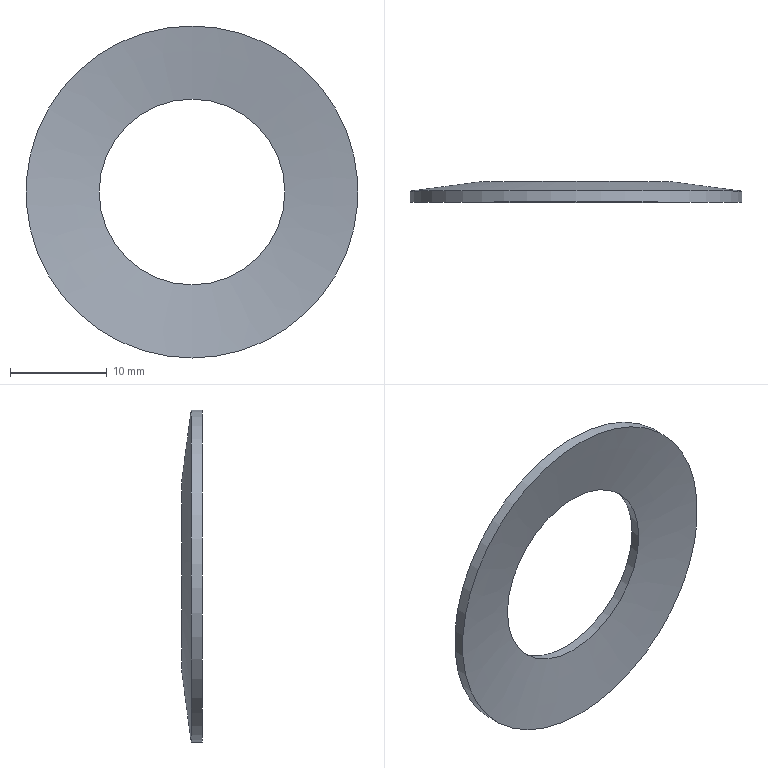Part | NX | features belleville 1.35in 2 | 1 solid | 4 faces | box 34.29 x 2.131 x 34.29 mm | volume 726.461 mm3 | cone 3 | cylinder 1 | commonest cylinder face diameters 34.29 x1
STEP:
#1=CARTESIAN_POINT('',(0.,0.2317,-17.145));
#2=VERTEX_POINT('',#1);
#3=CARTESIAN_POINT('',(0.,0.2317,0.));
#4=DIRECTION('',(0.,-1.,0.));
#5=DIRECTION('',(0.,0.,-1.));
#6=AXIS2_PLACEMENT_3D('',#3,#4,#5);
#7=CIRCLE('',#6,17.145);
#8=EDGE_CURVE('',#2,#2,#7,.F.);
#9=ORIENTED_EDGE('',*,*,#8,.F.);
#10=EDGE_LOOP('',(#9));
#11=FACE_BOUND('',#10,.T.);
#12=CARTESIAN_POINT('',(0.,1.229,-9.588));
#13=VERTEX_POINT('',#12);
#14=CARTESIAN_POINT('',(0.,1.229,0.));
#15=DIRECTION('',(0.,-1.,0.));
#16=DIRECTION('',(0.,0.,-1.));
#17=AXIS2_PLACEMENT_3D('',#14,#15,#16);
#18=CIRCLE('',#17,9.588);
#19=EDGE_CURVE('',#13,#13,#18,.T.);
#20=ORIENTED_EDGE('',*,*,#19,.F.);
#21=EDGE_LOOP('',(#20));
#22=FACE_BOUND('',#21,.T.);
#23=CARTESIAN_POINT('',(0.,1.229,0.));
#24=DIRECTION('',(0.,-1.,0.));
#25=DIRECTION('',(0.,0.,-1.));
#26=AXIS2_PLACEMENT_3D('',#23,#24,#25);
#27=CONICAL_SURFACE('',#26,9.588,1.44);
#28=ADVANCED_FACE('',(#11,#22),#27,.F.);
#29=ORIENTED_EDGE('',*,*,#19,.T.);
#30=EDGE_LOOP('',(#29));
#31=FACE_BOUND('',#30,.T.);
#32=CARTESIAN_POINT('',(0.,2.362,-9.738));
#33=VERTEX_POINT('',#32);
#34=CARTESIAN_POINT('',(0.,2.362,0.));
#35=DIRECTION('',(0.,-1.,0.));
#36=DIRECTION('',(0.,0.,-1.));
#37=AXIS2_PLACEMENT_3D('',#34,#35,#36);
#38=CIRCLE('',#37,9.738);
#39=EDGE_CURVE('',#33,#33,#38,.T.);
#40=ORIENTED_EDGE('',*,*,#39,.F.);
#41=EDGE_LOOP('',(#40));
#42=FACE_BOUND('',#41,.T.);
#43=CARTESIAN_POINT('',(0.,2.362,0.));
#44=DIRECTION('',(0.,1.,0.));
#45=DIRECTION('',(0.,0.,1.));
#46=AXIS2_PLACEMENT_3D('',#43,#44,#45);
#47=CONICAL_SURFACE('',#46,9.738,0.1312);
#48=ADVANCED_FACE('',(#31,#42),#47,.F.);
#49=CARTESIAN_POINT('',(0.,1.385,-17.145));
#50=VERTEX_POINT('',#49);
#51=CARTESIAN_POINT('',(0.,1.385,0.));
#52=DIRECTION('',(0.,-1.,0.));
#53=DIRECTION('',(0.,0.,-1.));
#54=AXIS2_PLACEMENT_3D('',#51,#52,#53);
#55=CIRCLE('',#54,17.145);
#56=EDGE_CURVE('',#50,#50,#55,.T.);
#57=ORIENTED_EDGE('',*,*,#56,.F.);
#58=EDGE_LOOP('',(#57));
#59=FACE_BOUND('',#58,.T.);
#60=ORIENTED_EDGE('',*,*,#39,.T.);
#61=EDGE_LOOP('',(#60));
#62=FACE_BOUND('',#61,.T.);
#63=CARTESIAN_POINT('',(0.,1.133,0.));
#64=DIRECTION('',(0.,-1.,0.));
#65=DIRECTION('',(0.,0.,-1.));
#66=AXIS2_PLACEMENT_3D('',#63,#64,#65);
#67=CONICAL_SURFACE('',#66,19.05,1.44);
#68=ADVANCED_FACE('',(#59,#62),#67,.T.);
#69=ORIENTED_EDGE('',*,*,#8,.T.);
#70=EDGE_LOOP('',(#69));
#71=FACE_BOUND('',#70,.T.);
#72=ORIENTED_EDGE('',*,*,#56,.T.);
#73=EDGE_LOOP('',(#72));
#74=FACE_BOUND('',#73,.T.);
#75=CARTESIAN_POINT('',(0.,2.362,0.));
#76=DIRECTION('',(0.,-1.,0.));
#77=DIRECTION('',(0.,0.,-1.));
#78=AXIS2_PLACEMENT_3D('',#75,#76,#77);
#79=CYLINDRICAL_SURFACE('',#78,17.145);
#80=ADVANCED_FACE('',(#71,#74),#79,.T.);
#81=CLOSED_SHELL('',(#28,#48,#68,#80));
#82=MANIFOLD_SOLID_BREP('',#81);
#83=(LENGTH_UNIT()NAMED_UNIT(*)SI_UNIT(.MILLI.,.METRE.));
#84=UNCERTAINTY_MEASURE_WITH_UNIT(LENGTH_MEASURE(0.00001),#83,'','');
#85=(NAMED_UNIT(*)PLANE_ANGLE_UNIT()SI_UNIT($,.RADIAN.));
#86=(NAMED_UNIT(*)SI_UNIT($,.STERADIAN.)SOLID_ANGLE_UNIT());
#87=(GEOMETRIC_REPRESENTATION_CONTEXT(3)GLOBAL_UNCERTAINTY_ASSIGNED_CONTEXT((#84))GLOBAL_UNIT_ASSIGNED_CONTEXT((#83,#85,#86))REPRESENTATION_CONTEXT('',''));
#88=ADVANCED_BREP_SHAPE_REPRESENTATION('',(#82),#87);